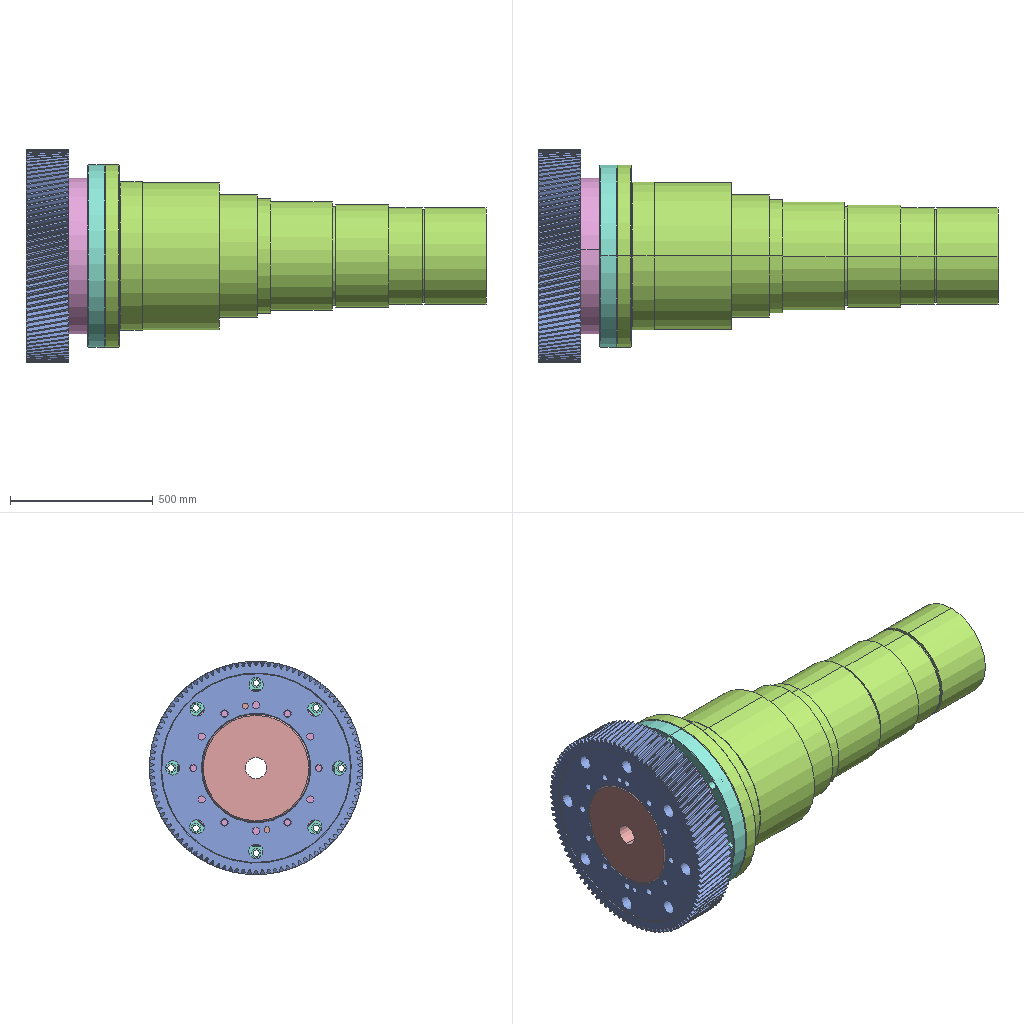Assembly | SolidWorks | 10 different items | 10 placed | box 1612 x 747 x 747 mm
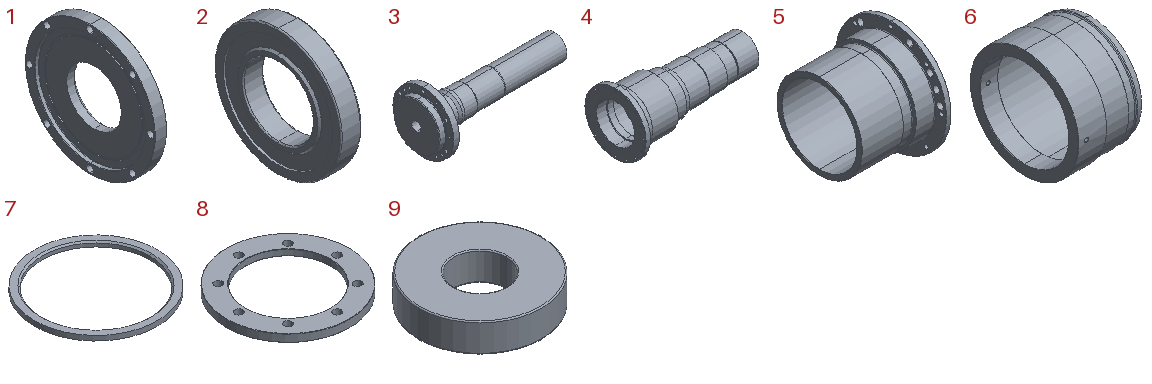Parts list (item | quantity | size | volume | features):
1 | x1 | 80 x 640 x 640 mm | 12908044 mm3 | features Chamfer 2, Fillet 2, ICE 2, Revolution 1
2 | x1 | 65 x 400 x 400 mm | 5037424 mm3 | features Revolution 5, Attribute 2, CirPattern 1, RefAxis 1
3 | x1 | 1136 x 500 x 500 mm | 46733705 mm3 | features ICE 2, 3DProfileFeature 1, HoleWzd 1, Revolution 1
4 | x1 | 1335 x 640 x 640 mm | 106671077 mm3 | features 3DProfileFeature 2, HoleWzd 2, ICE 2, Revolution 1
5 | x1 | 220 x 318 x 318 mm | 2874143 mm3 | features Chamfer 2, Fillet 2, ICE 2, Revolution 1
6 | x1 | 165 x 270 x 270 mm | 1639814 mm3 | features 3DProfileFeature 1, Chamfer 1, Fillet 1, HoleWzd 1, Revolution 1
7 | x1 | 252 x 252 x 10 mm | 115488 mm3 | features Chamfer 1, Extrusion 1
8 | x1 | 400 x 400 x 25 mm | 1378515 mm3 | features Chamfer 2, Extrusion 1, Fillet 1, ICE 1
9 | x1 | 546.1 x 546.1 x 127 mm | 24214209 mm3 | features Extrusion 1, Fillet 1
10 | x1 | - | - | features ICE 5, Boss 3, CirPattern 3, Fillet 3, Cut 2, Helix 2, SweepCut 2, 3DProfileFeature 1, Chamfer 1, HoleWzd 1, Revolution 1
Mates (type | each side: item.copy, entity, surface, feature):
Concentric | 3.1 face cylinder Revolve1 | 4.1 face cylinder Revolve1
Concentric | 3.1 face cylinder Revolve1 | 10.1 face cylinder Cut-Extrude1
Coincident | 3.1 face plane Revolve1 | 10.1 face plane Cut-Extrude4
Parallel | 3.1 face cylinder Cut-Extrude1 | 10.1 face cylinder Cut-Extrude5
Concentric | 3.1 face cylinder Revolve1 | 9.1 face cylinder Boss-Extrude1
Coincident | 3.1 face plane Revolve1 | 9.1 face plane Boss-Extrude1
Concentric | 9.1 face cylinder Boss-Extrude1 | 1.1 face cylinder Revolve1
Coincident | 9.1 face plane Boss-Extrude1 | 1.1 face plane Revolve1
Coincident | 4.1 face plane Revolve1 | 1.1 face plane Revolve1
Concentric | 3.1 face cylinder Revolve1 | 2.1 face cylinder InnerRace
Coincident | 1.1 face plane Revolve1 | 2.1 face plane OuterRace
Concentric | 3.1 face cylinder Revolve1 | 7.1 face cylinder Boss-Extrude1
Coincident | 3.1 face plane Revolve1 | 7.1 face plane Boss-Extrude1
Concentric | 5.1 face cylinder Revolve1 | 6.1 face cylinder Revolve1
Concentric | 3.1 face cylinder Revolve1 | 5.1 face cylinder Revolve1
Coincident | 2.1 face plane InnerRace | 6.1 face plane Revolve1
Concentric | 5.1 face cylinder Revolve1 | 4.1 edge
Coincident | 4.1 edge | 5.1 face plane Revolve1
Coincident | 2.1 face plane OuterRace | 8.1 face plane Boss-Extrude1
Concentric | 4.1 face cylinder Revolve1 | 8.1 face cylinder Boss-Extrude1
Parallel | 3.1 select_type:24 | 8.1 select_type:24
Parallel | 3.1 select_type:24 | 6.1 select_type:24
Concentric | 4.1 face cylinder Cut-Extrude2 | 1.1 face cylinder Cut-Extrude2
Parallel | 3.1 select_type:24 | 4.1 select_type:24
Parallel | 3.1 select_type:24 | 5.1 select_type:24